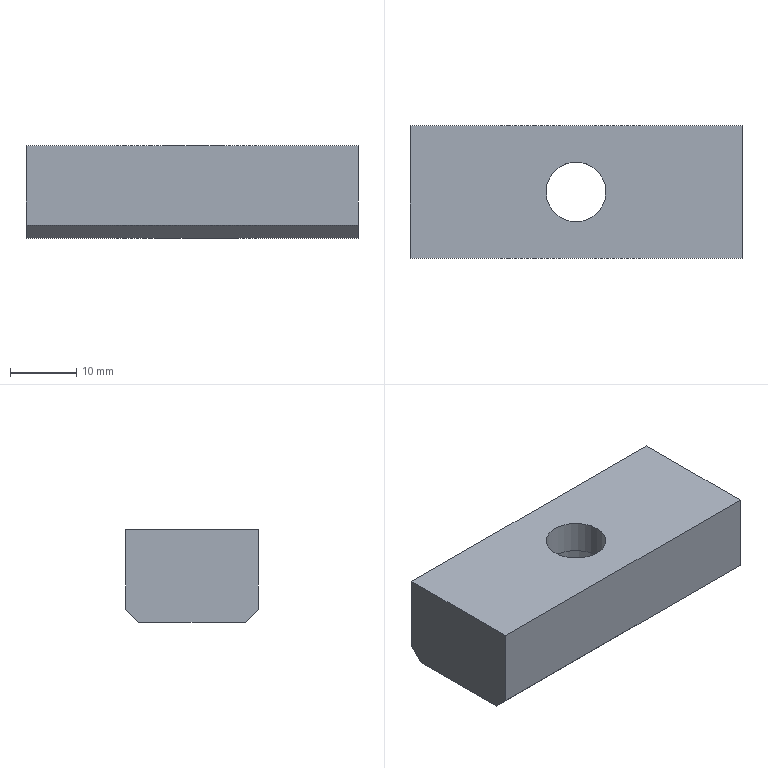Part | NX | features solid 2 | 1 solid | 11 faces | box 50 x 20 x 14 mm | volume 12096 mm3 | plane 9 | cylinder 2 | commonest cylinder face diameters 9 x1 14 x1
STEP:
#1=CARTESIAN_POINT('',(424.,-287.,66.));
#2=VERTEX_POINT('',#1);
#3=CARTESIAN_POINT('',(424.,-287.,78.));
#4=VERTEX_POINT('',#3);
#5=CARTESIAN_POINT('',(424.,-287.,64.));
#6=DIRECTION('',(0.,0.,1.));
#7=VECTOR('',#6,1000.);
#8=LINE('',#5,#7);
#9=EDGE_CURVE('',#2,#4,#8,.T.);
#10=ORIENTED_EDGE('',*,*,#9,.T.);
#11=CARTESIAN_POINT('',(374.,-287.,78.));
#12=VERTEX_POINT('',#11);
#13=CARTESIAN_POINT('',(374.,-287.,78.));
#14=DIRECTION('',(-1.,0.,0.));
#15=VECTOR('',#14,1000.);
#16=LINE('',#13,#15);
#17=EDGE_CURVE('',#12,#4,#16,.F.);
#18=ORIENTED_EDGE('',*,*,#17,.F.);
#19=CARTESIAN_POINT('',(374.,-287.,66.));
#20=VERTEX_POINT('',#19);
#21=CARTESIAN_POINT('',(374.,-287.,64.));
#22=DIRECTION('',(0.,0.,1.));
#23=VECTOR('',#22,1000.);
#24=LINE('',#21,#23);
#25=EDGE_CURVE('',#20,#12,#24,.T.);
#26=ORIENTED_EDGE('',*,*,#25,.F.);
#27=CARTESIAN_POINT('',(374.,-287.,66.));
#28=DIRECTION('',(-1.,0.,0.));
#29=VECTOR('',#28,1000.);
#30=LINE('',#27,#29);
#31=EDGE_CURVE('',#2,#20,#30,.T.);
#32=ORIENTED_EDGE('',*,*,#31,.F.);
#33=EDGE_LOOP('',(#10,#18,#26,#32));
#34=FACE_BOUND('',#33,.T.);
#35=CARTESIAN_POINT('',(374.,-287.,64.));
#36=DIRECTION('',(0.,-1.,0.));
#37=DIRECTION('',(1.,0.,0.));
#38=AXIS2_PLACEMENT_3D('',#35,#36,#37);
#39=PLANE('',#38);
#40=ADVANCED_FACE('',(#34),#39,.T.);
#41=ORIENTED_EDGE('',*,*,#25,.T.);
#42=CARTESIAN_POINT('',(374.,-267.,78.));
#43=VERTEX_POINT('',#42);
#44=CARTESIAN_POINT('',(374.,-287.,78.));
#45=DIRECTION('',(0.,-1.,0.));
#46=VECTOR('',#45,1000.);
#47=LINE('',#44,#46);
#48=EDGE_CURVE('',#12,#43,#47,.F.);
#49=ORIENTED_EDGE('',*,*,#48,.T.);
#50=CARTESIAN_POINT('',(374.,-267.,66.));
#51=VERTEX_POINT('',#50);
#52=CARTESIAN_POINT('',(374.,-267.,64.));
#53=DIRECTION('',(0.,0.,1.));
#54=VECTOR('',#53,1000.);
#55=LINE('',#52,#54);
#56=EDGE_CURVE('',#51,#43,#55,.T.);
#57=ORIENTED_EDGE('',*,*,#56,.F.);
#58=CARTESIAN_POINT('',(374.,-269.,64.));
#59=VERTEX_POINT('',#58);
#60=CARTESIAN_POINT('',(374.,-278.,55.));
#61=DIRECTION('',(0.,-0.7071,-0.7071));
#62=VECTOR('',#61,1000.);
#63=LINE('',#60,#62);
#64=EDGE_CURVE('',#59,#51,#63,.F.);
#65=ORIENTED_EDGE('',*,*,#64,.F.);
#66=CARTESIAN_POINT('',(374.,-285.,64.));
#67=VERTEX_POINT('',#66);
#68=CARTESIAN_POINT('',(374.,-287.,64.));
#69=DIRECTION('',(0.,1.,0.));
#70=VECTOR('',#69,1000.);
#71=LINE('',#68,#70);
#72=EDGE_CURVE('',#67,#59,#71,.T.);
#73=ORIENTED_EDGE('',*,*,#72,.F.);
#74=CARTESIAN_POINT('',(374.,-286.,65.));
#75=DIRECTION('',(0.,0.7071,-0.7071));
#76=VECTOR('',#75,1000.);
#77=LINE('',#74,#76);
#78=EDGE_CURVE('',#20,#67,#77,.T.);
#79=ORIENTED_EDGE('',*,*,#78,.F.);
#80=EDGE_LOOP('',(#41,#49,#57,#65,#73,#79));
#81=FACE_BOUND('',#80,.T.);
#82=CARTESIAN_POINT('',(374.,-287.,64.));
#83=DIRECTION('',(1.,0.,0.));
#84=DIRECTION('',(0.,1.,0.));
#85=AXIS2_PLACEMENT_3D('',#82,#83,#84);
#86=PLANE('',#85);
#87=ADVANCED_FACE('',(#81),#86,.F.);
#88=ORIENTED_EDGE('',*,*,#56,.T.);
#89=CARTESIAN_POINT('',(424.,-267.,78.));
#90=VERTEX_POINT('',#89);
#91=CARTESIAN_POINT('',(374.,-267.,78.));
#92=DIRECTION('',(-1.,0.,0.));
#93=VECTOR('',#92,1000.);
#94=LINE('',#91,#93);
#95=EDGE_CURVE('',#43,#90,#94,.F.);
#96=ORIENTED_EDGE('',*,*,#95,.T.);
#97=CARTESIAN_POINT('',(424.,-267.,66.));
#98=VERTEX_POINT('',#97);
#99=CARTESIAN_POINT('',(424.,-267.,64.));
#100=DIRECTION('',(0.,0.,1.));
#101=VECTOR('',#100,1000.);
#102=LINE('',#99,#101);
#103=EDGE_CURVE('',#98,#90,#102,.T.);
#104=ORIENTED_EDGE('',*,*,#103,.F.);
#105=CARTESIAN_POINT('',(374.,-267.,66.));
#106=DIRECTION('',(-1.,0.,0.));
#107=VECTOR('',#106,1000.);
#108=LINE('',#105,#107);
#109=EDGE_CURVE('',#51,#98,#108,.F.);
#110=ORIENTED_EDGE('',*,*,#109,.F.);
#111=EDGE_LOOP('',(#88,#96,#104,#110));
#112=FACE_BOUND('',#111,.T.);
#113=CARTESIAN_POINT('',(374.,-267.,64.));
#114=DIRECTION('',(0.,-1.,0.));
#115=DIRECTION('',(1.,0.,0.));
#116=AXIS2_PLACEMENT_3D('',#113,#114,#115);
#117=PLANE('',#116);
#118=ADVANCED_FACE('',(#112),#117,.F.);
#119=CARTESIAN_POINT('',(424.,-285.,64.));
#120=VERTEX_POINT('',#119);
#121=CARTESIAN_POINT('',(424.,-269.,64.));
#122=VERTEX_POINT('',#121);
#123=CARTESIAN_POINT('',(424.,-287.,64.));
#124=DIRECTION('',(0.,1.,0.));
#125=VECTOR('',#124,1000.);
#126=LINE('',#123,#125);
#127=EDGE_CURVE('',#120,#122,#126,.T.);
#128=ORIENTED_EDGE('',*,*,#127,.T.);
#129=CARTESIAN_POINT('',(424.,-278.,55.));
#130=DIRECTION('',(0.,-0.7071,-0.7071));
#131=VECTOR('',#130,1000.);
#132=LINE('',#129,#131);
#133=EDGE_CURVE('',#98,#122,#132,.T.);
#134=ORIENTED_EDGE('',*,*,#133,.F.);
#135=ORIENTED_EDGE('',*,*,#103,.T.);
#136=CARTESIAN_POINT('',(424.,-287.,78.));
#137=DIRECTION('',(0.,-1.,0.));
#138=VECTOR('',#137,1000.);
#139=LINE('',#136,#138);
#140=EDGE_CURVE('',#4,#90,#139,.F.);
#141=ORIENTED_EDGE('',*,*,#140,.F.);
#142=ORIENTED_EDGE('',*,*,#9,.F.);
#143=CARTESIAN_POINT('',(424.,-286.,65.));
#144=DIRECTION('',(0.,0.7071,-0.7071));
#145=VECTOR('',#144,1000.);
#146=LINE('',#143,#145);
#147=EDGE_CURVE('',#120,#2,#146,.F.);
#148=ORIENTED_EDGE('',*,*,#147,.F.);
#149=EDGE_LOOP('',(#128,#134,#135,#141,#142,#148));
#150=FACE_BOUND('',#149,.T.);
#151=CARTESIAN_POINT('',(424.,-287.,64.));
#152=DIRECTION('',(1.,0.,0.));
#153=DIRECTION('',(0.,1.,0.));
#154=AXIS2_PLACEMENT_3D('',#151,#152,#153);
#155=PLANE('',#154);
#156=ADVANCED_FACE('',(#150),#155,.T.);
#157=CARTESIAN_POINT('',(394.5,-277.,78.));
#158=VERTEX_POINT('',#157);
#159=CARTESIAN_POINT('',(399.,-277.,78.));
#160=DIRECTION('',(0.,0.,1.));
#161=DIRECTION('',(-1.,0.,0.));
#162=AXIS2_PLACEMENT_3D('',#159,#160,#161);
#163=CIRCLE('',#162,4.5);
#164=EDGE_CURVE('',#158,#158,#163,.T.);
#165=ORIENTED_EDGE('',*,*,#164,.F.);
#166=EDGE_LOOP('',(#165));
#167=FACE_BOUND('',#166,.T.);
#168=ORIENTED_EDGE('',*,*,#95,.F.);
#169=ORIENTED_EDGE('',*,*,#48,.F.);
#170=ORIENTED_EDGE('',*,*,#17,.T.);
#171=ORIENTED_EDGE('',*,*,#140,.T.);
#172=EDGE_LOOP('',(#168,#169,#170,#171));
#173=FACE_BOUND('',#172,.T.);
#174=CARTESIAN_POINT('',(374.,-287.,78.));
#175=DIRECTION('',(0.,0.,-1.));
#176=DIRECTION('',(-1.,0.,0.));
#177=AXIS2_PLACEMENT_3D('',#174,#175,#176);
#178=PLANE('',#177);
#179=ADVANCED_FACE('',(#167,#173),#178,.F.);
#180=CARTESIAN_POINT('',(406.,-277.,64.));
#181=VERTEX_POINT('',#180);
#182=CARTESIAN_POINT('',(399.,-277.,64.));
#183=DIRECTION('',(0.,0.,-1.));
#184=DIRECTION('',(1.,0.,0.));
#185=AXIS2_PLACEMENT_3D('',#182,#183,#184);
#186=CIRCLE('',#185,7.);
#187=EDGE_CURVE('',#181,#181,#186,.T.);
#188=ORIENTED_EDGE('',*,*,#187,.F.);
#189=EDGE_LOOP('',(#188));
#190=FACE_BOUND('',#189,.T.);
#191=ORIENTED_EDGE('',*,*,#72,.T.);
#192=CARTESIAN_POINT('',(374.,-269.,64.));
#193=DIRECTION('',(-1.,0.,0.));
#194=VECTOR('',#193,1000.);
#195=LINE('',#192,#194);
#196=EDGE_CURVE('',#122,#59,#195,.T.);
#197=ORIENTED_EDGE('',*,*,#196,.F.);
#198=ORIENTED_EDGE('',*,*,#127,.F.);
#199=CARTESIAN_POINT('',(374.,-285.,64.));
#200=DIRECTION('',(1.,0.,0.));
#201=VECTOR('',#200,1000.);
#202=LINE('',#199,#201);
#203=EDGE_CURVE('',#67,#120,#202,.T.);
#204=ORIENTED_EDGE('',*,*,#203,.F.);
#205=EDGE_LOOP('',(#191,#197,#198,#204));
#206=FACE_BOUND('',#205,.T.);
#207=CARTESIAN_POINT('',(374.,-287.,64.));
#208=DIRECTION('',(0.,0.,-1.));
#209=DIRECTION('',(-1.,0.,0.));
#210=AXIS2_PLACEMENT_3D('',#207,#208,#209);
#211=PLANE('',#210);
#212=ADVANCED_FACE('',(#190,#206),#211,.T.);
#213=ORIENTED_EDGE('',*,*,#78,.T.);
#214=ORIENTED_EDGE('',*,*,#203,.T.);
#215=ORIENTED_EDGE('',*,*,#147,.T.);
#216=ORIENTED_EDGE('',*,*,#31,.T.);
#217=EDGE_LOOP('',(#213,#214,#215,#216));
#218=FACE_BOUND('',#217,.T.);
#219=CARTESIAN_POINT('',(374.,-285.,64.));
#220=DIRECTION('',(0.,0.7071,0.7071));
#221=DIRECTION('',(0.,0.7071,-0.7071));
#222=AXIS2_PLACEMENT_3D('',#219,#220,#221);
#223=PLANE('',#222);
#224=ADVANCED_FACE('',(#218),#223,.F.);
#225=ORIENTED_EDGE('',*,*,#64,.T.);
#226=ORIENTED_EDGE('',*,*,#109,.T.);
#227=ORIENTED_EDGE('',*,*,#133,.T.);
#228=ORIENTED_EDGE('',*,*,#196,.T.);
#229=EDGE_LOOP('',(#225,#226,#227,#228));
#230=FACE_BOUND('',#229,.T.);
#231=CARTESIAN_POINT('',(374.,-267.,66.));
#232=DIRECTION('',(0.,0.7071,-0.7071));
#233=DIRECTION('',(0.,-0.7071,-0.7071));
#234=AXIS2_PLACEMENT_3D('',#231,#232,#233);
#235=PLANE('',#234);
#236=ADVANCED_FACE('',(#230),#235,.T.);
#237=ORIENTED_EDGE('',*,*,#187,.T.);
#238=EDGE_LOOP('',(#237));
#239=FACE_BOUND('',#238,.T.);
#240=CARTESIAN_POINT('',(406.,-277.,73.));
#241=VERTEX_POINT('',#240);
#242=CARTESIAN_POINT('',(399.,-277.,73.));
#243=DIRECTION('',(0.,0.,-1.));
#244=DIRECTION('',(1.,0.,0.));
#245=AXIS2_PLACEMENT_3D('',#242,#243,#244);
#246=CIRCLE('',#245,7.);
#247=EDGE_CURVE('',#241,#241,#246,.T.);
#248=ORIENTED_EDGE('',*,*,#247,.F.);
#249=EDGE_LOOP('',(#248));
#250=FACE_BOUND('',#249,.T.);
#251=CARTESIAN_POINT('',(399.,-277.,64.));
#252=DIRECTION('',(0.,0.,1.));
#253=DIRECTION('',(1.,0.,0.));
#254=AXIS2_PLACEMENT_3D('',#251,#252,#253);
#255=CYLINDRICAL_SURFACE('',#254,7.);
#256=ADVANCED_FACE('',(#239,#250),#255,.F.);
#257=CARTESIAN_POINT('',(403.5,-277.,73.));
#258=VERTEX_POINT('',#257);
#259=CARTESIAN_POINT('',(399.,-277.,73.));
#260=DIRECTION('',(0.,0.,-1.));
#261=DIRECTION('',(1.,0.,0.));
#262=AXIS2_PLACEMENT_3D('',#259,#260,#261);
#263=CIRCLE('',#262,4.5);
#264=EDGE_CURVE('',#258,#258,#263,.T.);
#265=ORIENTED_EDGE('',*,*,#264,.F.);
#266=EDGE_LOOP('',(#265));
#267=FACE_BOUND('',#266,.T.);
#268=ORIENTED_EDGE('',*,*,#247,.T.);
#269=EDGE_LOOP('',(#268));
#270=FACE_BOUND('',#269,.T.);
#271=CARTESIAN_POINT('',(399.,-277.,73.));
#272=DIRECTION('',(0.,0.,1.));
#273=DIRECTION('',(1.,0.,0.));
#274=AXIS2_PLACEMENT_3D('',#271,#272,#273);
#275=PLANE('',#274);
#276=ADVANCED_FACE('',(#267,#270),#275,.F.);
#277=ORIENTED_EDGE('',*,*,#264,.T.);
#278=EDGE_LOOP('',(#277));
#279=FACE_BOUND('',#278,.T.);
#280=ORIENTED_EDGE('',*,*,#164,.T.);
#281=EDGE_LOOP('',(#280));
#282=FACE_BOUND('',#281,.T.);
#283=CARTESIAN_POINT('',(399.,-277.,64.));
#284=DIRECTION('',(0.,0.,1.));
#285=DIRECTION('',(1.,0.,0.));
#286=AXIS2_PLACEMENT_3D('',#283,#284,#285);
#287=CYLINDRICAL_SURFACE('',#286,4.5);
#288=ADVANCED_FACE('',(#279,#282),#287,.F.);
#289=CLOSED_SHELL('',(#40,#87,#118,#156,#179,#212,#224,#236,#256,#276,#288));
#290=MANIFOLD_SOLID_BREP('',#289);
#291=(LENGTH_UNIT()NAMED_UNIT(*)SI_UNIT(.MILLI.,.METRE.));
#292=UNCERTAINTY_MEASURE_WITH_UNIT(LENGTH_MEASURE(0.00001),#291,'','');
#293=(NAMED_UNIT(*)PLANE_ANGLE_UNIT()SI_UNIT($,.RADIAN.));
#294=(NAMED_UNIT(*)SI_UNIT($,.STERADIAN.)SOLID_ANGLE_UNIT());
#295=(GEOMETRIC_REPRESENTATION_CONTEXT(3)GLOBAL_UNCERTAINTY_ASSIGNED_CONTEXT((#292))GLOBAL_UNIT_ASSIGNED_CONTEXT((#291,#293,#294))REPRESENTATION_CONTEXT('',''));
#296=ADVANCED_BREP_SHAPE_REPRESENTATION('',(#290),#295);